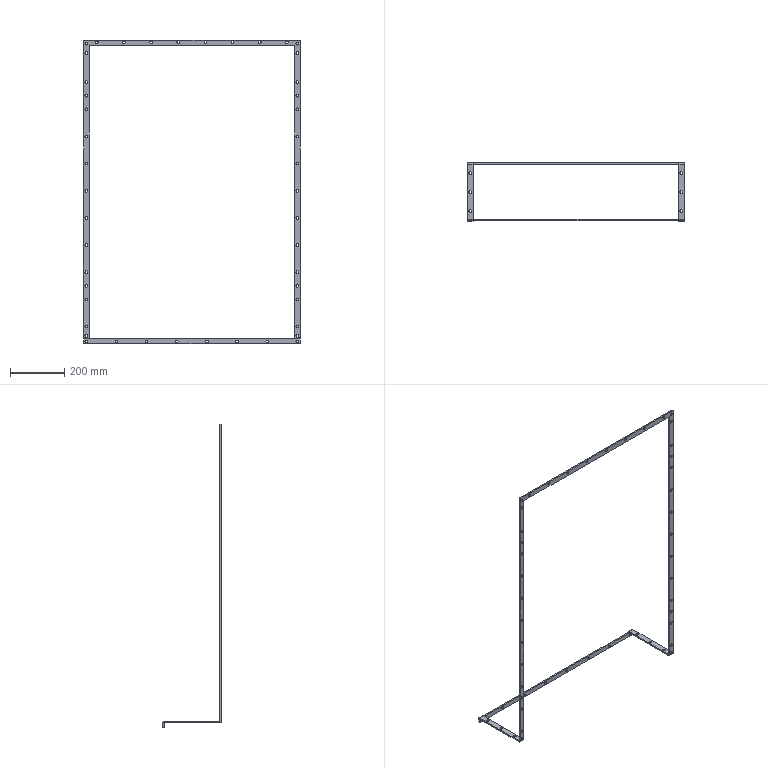Part | NX | features BREP 1 | 1 solid | 128 faces | box 798.203 x 215.5 x 1117 mm | volume 386704 mm3 | cylinder 112 | plane 16 | commonest cylinder face diameters 10 x112